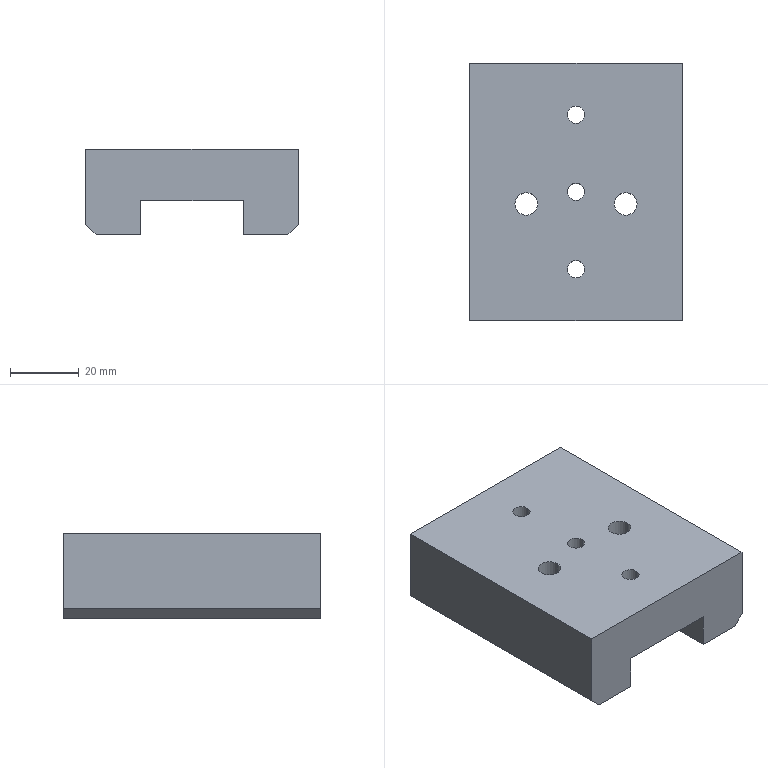Part | SolidWorks | features HoleWzd 3, Chamfer 1, Extrusion 1, ICE 1 | 1 solid | 30 faces | box 62 x 75 x 25 mm | volume 89108 mm3 | plane 16 | cylinder 14 | commonest cylinder face diameters 5 x6 6.6 x4 11 x4
STEP:
#1=CARTESIAN_POINT('',(17.8,-3.5,12.5));
#2=VERTEX_POINT('',#1);
#3=CARTESIAN_POINT('',(11.2,-3.5,12.5));
#4=VERTEX_POINT('',#3);
#5=CARTESIAN_POINT('',(14.5,-3.5,12.5));
#6=DIRECTION('',(0.,0.,-1.));
#7=DIRECTION('',(-1.,0.,0.));
#8=AXIS2_PLACEMENT_3D('',#5,#6,#7);
#9=CIRCLE('',#8,3.3);
#10=EDGE_CURVE('',#2,#4,#9,.T.);
#11=ORIENTED_EDGE('',*,*,#10,.F.);
#12=CARTESIAN_POINT('',(17.8,-3.5,7.5));
#13=VERTEX_POINT('',#12);
#14=CARTESIAN_POINT('',(17.8,-3.5,-12.5));
#15=DIRECTION('',(0.,0.,-1.));
#16=VECTOR('',#15,1000.);
#17=LINE('',#14,#16);
#18=EDGE_CURVE('',#2,#13,#17,.T.);
#19=ORIENTED_EDGE('',*,*,#18,.T.);
#20=CARTESIAN_POINT('',(11.2,-3.5,7.5));
#21=VERTEX_POINT('',#20);
#22=CARTESIAN_POINT('',(14.5,-3.5,7.5));
#23=DIRECTION('',(0.,0.,-1.));
#24=DIRECTION('',(-1.,0.,0.));
#25=AXIS2_PLACEMENT_3D('',#22,#23,#24);
#26=CIRCLE('',#25,3.3);
#27=EDGE_CURVE('',#13,#21,#26,.T.);
#28=ORIENTED_EDGE('',*,*,#27,.T.);
#29=CARTESIAN_POINT('',(11.2,-3.5,-12.5));
#30=DIRECTION('',(0.,0.,-1.));
#31=VECTOR('',#30,1000.);
#32=LINE('',#29,#31);
#33=EDGE_CURVE('',#4,#21,#32,.T.);
#34=ORIENTED_EDGE('',*,*,#33,.F.);
#35=EDGE_LOOP('',(#11,#19,#28,#34));
#36=FACE_OUTER_BOUND('',#35,.T.);
#37=CARTESIAN_POINT('',(14.5,-3.5,-12.5));
#38=DIRECTION('',(0.,0.,-1.));
#39=DIRECTION('',(-1.,0.,0.));
#40=AXIS2_PLACEMENT_3D('',#37,#38,#39);
#41=CYLINDRICAL_SURFACE('',#40,3.3);
#42=ADVANCED_FACE('',(#36),#41,.F.);
#43=CARTESIAN_POINT('',(20.,-3.5,7.5));
#44=VERTEX_POINT('',#43);
#45=CARTESIAN_POINT('',(9.,-3.5,7.5));
#46=VERTEX_POINT('',#45);
#47=CARTESIAN_POINT('',(14.5,-3.5,7.5));
#48=DIRECTION('',(0.,0.,-1.));
#49=DIRECTION('',(-1.,0.,0.));
#50=AXIS2_PLACEMENT_3D('',#47,#48,#49);
#51=CIRCLE('',#50,5.5);
#52=EDGE_CURVE('',#44,#46,#51,.T.);
#53=ORIENTED_EDGE('',*,*,#52,.F.);
#54=CARTESIAN_POINT('',(20.,-3.5,-12.5));
#55=VERTEX_POINT('',#54);
#56=CARTESIAN_POINT('',(20.,-3.5,-12.5));
#57=DIRECTION('',(0.,0.,-1.));
#58=VECTOR('',#57,1000.);
#59=LINE('',#56,#58);
#60=EDGE_CURVE('',#44,#55,#59,.T.);
#61=ORIENTED_EDGE('',*,*,#60,.T.);
#62=CARTESIAN_POINT('',(15.,-8.977,-12.5));
#63=VERTEX_POINT('',#62);
#64=CARTESIAN_POINT('',(14.5,-3.5,-12.5));
#65=DIRECTION('',(0.,0.,-1.));
#66=DIRECTION('',(-1.,0.,0.));
#67=AXIS2_PLACEMENT_3D('',#64,#65,#66);
#68=CIRCLE('',#67,5.5);
#69=EDGE_CURVE('',#55,#63,#68,.T.);
#70=ORIENTED_EDGE('',*,*,#69,.T.);
#71=CARTESIAN_POINT('',(15.,-8.977,-2.5));
#72=VERTEX_POINT('',#71);
#73=CARTESIAN_POINT('',(15.,-8.977,-12.5));
#74=DIRECTION('',(0.,0.,-1.));
#75=VECTOR('',#74,1000.);
#76=LINE('',#73,#75);
#77=EDGE_CURVE('',#72,#63,#76,.T.);
#78=ORIENTED_EDGE('',*,*,#77,.F.);
#79=CARTESIAN_POINT('',(9.,-3.5,-2.5));
#80=VERTEX_POINT('',#79);
#81=CARTESIAN_POINT('',(14.5,-3.5,-2.5));
#82=DIRECTION('',(0.,0.,-1.));
#83=DIRECTION('',(-1.,0.,0.));
#84=AXIS2_PLACEMENT_3D('',#81,#82,#83);
#85=CIRCLE('',#84,5.5);
#86=EDGE_CURVE('',#72,#80,#85,.T.);
#87=ORIENTED_EDGE('',*,*,#86,.T.);
#88=CARTESIAN_POINT('',(9.,-3.5,-12.5));
#89=DIRECTION('',(0.,0.,-1.));
#90=VECTOR('',#89,1000.);
#91=LINE('',#88,#90);
#92=EDGE_CURVE('',#46,#80,#91,.T.);
#93=ORIENTED_EDGE('',*,*,#92,.F.);
#94=EDGE_LOOP('',(#53,#61,#70,#78,#87,#93));
#95=FACE_OUTER_BOUND('',#94,.T.);
#96=CARTESIAN_POINT('',(14.5,-3.5,-12.5));
#97=DIRECTION('',(0.,0.,-1.));
#98=DIRECTION('',(-1.,0.,0.));
#99=AXIS2_PLACEMENT_3D('',#96,#97,#98);
#100=CYLINDRICAL_SURFACE('',#99,5.5);
#101=ADVANCED_FACE('',(#95),#100,.F.);
#102=CARTESIAN_POINT('',(-11.2,-3.5,12.5));
#103=VERTEX_POINT('',#102);
#104=CARTESIAN_POINT('',(-17.8,-3.5,12.5));
#105=VERTEX_POINT('',#104);
#106=CARTESIAN_POINT('',(-14.5,-3.5,12.5));
#107=DIRECTION('',(0.,0.,-1.));
#108=DIRECTION('',(-1.,0.,0.));
#109=AXIS2_PLACEMENT_3D('',#106,#107,#108);
#110=CIRCLE('',#109,3.3);
#111=EDGE_CURVE('',#103,#105,#110,.T.);
#112=ORIENTED_EDGE('',*,*,#111,.F.);
#113=CARTESIAN_POINT('',(-11.2,-3.5,7.5));
#114=VERTEX_POINT('',#113);
#115=CARTESIAN_POINT('',(-11.2,-3.5,-12.5));
#116=DIRECTION('',(0.,0.,-1.));
#117=VECTOR('',#116,1000.);
#118=LINE('',#115,#117);
#119=EDGE_CURVE('',#103,#114,#118,.T.);
#120=ORIENTED_EDGE('',*,*,#119,.T.);
#121=CARTESIAN_POINT('',(-17.8,-3.5,7.5));
#122=VERTEX_POINT('',#121);
#123=CARTESIAN_POINT('',(-14.5,-3.5,7.5));
#124=DIRECTION('',(0.,0.,-1.));
#125=DIRECTION('',(-1.,0.,0.));
#126=AXIS2_PLACEMENT_3D('',#123,#124,#125);
#127=CIRCLE('',#126,3.3);
#128=EDGE_CURVE('',#114,#122,#127,.T.);
#129=ORIENTED_EDGE('',*,*,#128,.T.);
#130=CARTESIAN_POINT('',(-17.8,-3.5,-12.5));
#131=DIRECTION('',(0.,0.,-1.));
#132=VECTOR('',#131,1000.);
#133=LINE('',#130,#132);
#134=EDGE_CURVE('',#105,#122,#133,.T.);
#135=ORIENTED_EDGE('',*,*,#134,.F.);
#136=EDGE_LOOP('',(#112,#120,#129,#135));
#137=FACE_OUTER_BOUND('',#136,.T.);
#138=CARTESIAN_POINT('',(-14.5,-3.5,-12.5));
#139=DIRECTION('',(0.,0.,-1.));
#140=DIRECTION('',(-1.,0.,0.));
#141=AXIS2_PLACEMENT_3D('',#138,#139,#140);
#142=CYLINDRICAL_SURFACE('',#141,3.3);
#143=ADVANCED_FACE('',(#137),#142,.F.);
#144=CARTESIAN_POINT('',(-9.,-3.5,7.5));
#145=VERTEX_POINT('',#144);
#146=CARTESIAN_POINT('',(-20.,-3.5,7.5));
#147=VERTEX_POINT('',#146);
#148=CARTESIAN_POINT('',(-14.5,-3.5,7.5));
#149=DIRECTION('',(0.,0.,-1.));
#150=DIRECTION('',(-1.,0.,0.));
#151=AXIS2_PLACEMENT_3D('',#148,#149,#150);
#152=CIRCLE('',#151,5.5);
#153=EDGE_CURVE('',#145,#147,#152,.T.);
#154=ORIENTED_EDGE('',*,*,#153,.F.);
#155=CARTESIAN_POINT('',(-9.,-3.5,-2.5));
#156=VERTEX_POINT('',#155);
#157=CARTESIAN_POINT('',(-9.,-3.5,-12.5));
#158=DIRECTION('',(0.,0.,-1.));
#159=VECTOR('',#158,1000.);
#160=LINE('',#157,#159);
#161=EDGE_CURVE('',#145,#156,#160,.T.);
#162=ORIENTED_EDGE('',*,*,#161,.T.);
#163=CARTESIAN_POINT('',(-15.,-8.977,-2.5));
#164=VERTEX_POINT('',#163);
#165=CARTESIAN_POINT('',(-14.5,-3.5,-2.5));
#166=DIRECTION('',(0.,0.,-1.));
#167=DIRECTION('',(-1.,0.,0.));
#168=AXIS2_PLACEMENT_3D('',#165,#166,#167);
#169=CIRCLE('',#168,5.5);
#170=EDGE_CURVE('',#156,#164,#169,.T.);
#171=ORIENTED_EDGE('',*,*,#170,.T.);
#172=CARTESIAN_POINT('',(-15.,-8.977,-12.5));
#173=VERTEX_POINT('',#172);
#174=CARTESIAN_POINT('',(-15.,-8.977,-12.5));
#175=DIRECTION('',(0.,0.,1.));
#176=VECTOR('',#175,1000.);
#177=LINE('',#174,#176);
#178=EDGE_CURVE('',#173,#164,#177,.T.);
#179=ORIENTED_EDGE('',*,*,#178,.F.);
#180=CARTESIAN_POINT('',(-20.,-3.5,-12.5));
#181=VERTEX_POINT('',#180);
#182=CARTESIAN_POINT('',(-14.5,-3.5,-12.5));
#183=DIRECTION('',(0.,0.,-1.));
#184=DIRECTION('',(-1.,0.,0.));
#185=AXIS2_PLACEMENT_3D('',#182,#183,#184);
#186=CIRCLE('',#185,5.5);
#187=EDGE_CURVE('',#173,#181,#186,.T.);
#188=ORIENTED_EDGE('',*,*,#187,.T.);
#189=CARTESIAN_POINT('',(-20.,-3.5,-12.5));
#190=DIRECTION('',(0.,0.,-1.));
#191=VECTOR('',#190,1000.);
#192=LINE('',#189,#191);
#193=EDGE_CURVE('',#147,#181,#192,.T.);
#194=ORIENTED_EDGE('',*,*,#193,.F.);
#195=EDGE_LOOP('',(#154,#162,#171,#179,#188,#194));
#196=FACE_OUTER_BOUND('',#195,.T.);
#197=CARTESIAN_POINT('',(-14.5,-3.5,-12.5));
#198=DIRECTION('',(0.,0.,-1.));
#199=DIRECTION('',(-1.,0.,0.));
#200=AXIS2_PLACEMENT_3D('',#197,#198,#199);
#201=CYLINDRICAL_SURFACE('',#200,5.5);
#202=ADVANCED_FACE('',(#196),#201,.F.);
#203=CARTESIAN_POINT('',(2.5,22.5,12.5));
#204=VERTEX_POINT('',#203);
#205=CARTESIAN_POINT('',(-2.5,22.5,12.5));
#206=VERTEX_POINT('',#205);
#207=CARTESIAN_POINT('',(0.,22.5,12.5));
#208=DIRECTION('',(0.,0.,-1.));
#209=DIRECTION('',(-1.,0.,0.));
#210=AXIS2_PLACEMENT_3D('',#207,#208,#209);
#211=CIRCLE('',#210,2.5);
#212=EDGE_CURVE('',#204,#206,#211,.T.);
#213=ORIENTED_EDGE('',*,*,#212,.F.);
#214=CARTESIAN_POINT('',(2.5,22.5,-2.5));
#215=VERTEX_POINT('',#214);
#216=CARTESIAN_POINT('',(2.5,22.5,-2.5));
#217=DIRECTION('',(0.,0.,-1.));
#218=VECTOR('',#217,1000.);
#219=LINE('',#216,#218);
#220=EDGE_CURVE('',#204,#215,#219,.T.);
#221=ORIENTED_EDGE('',*,*,#220,.T.);
#222=CARTESIAN_POINT('',(-2.5,22.5,-2.5));
#223=VERTEX_POINT('',#222);
#224=CARTESIAN_POINT('',(0.,22.5,-2.5));
#225=DIRECTION('',(0.,0.,-1.));
#226=DIRECTION('',(-1.,0.,0.));
#227=AXIS2_PLACEMENT_3D('',#224,#225,#226);
#228=CIRCLE('',#227,2.5);
#229=EDGE_CURVE('',#215,#223,#228,.T.);
#230=ORIENTED_EDGE('',*,*,#229,.T.);
#231=CARTESIAN_POINT('',(-2.5,22.5,-2.5));
#232=DIRECTION('',(0.,0.,-1.));
#233=VECTOR('',#232,1000.);
#234=LINE('',#231,#233);
#235=EDGE_CURVE('',#206,#223,#234,.T.);
#236=ORIENTED_EDGE('',*,*,#235,.F.);
#237=EDGE_LOOP('',(#213,#221,#230,#236));
#238=FACE_OUTER_BOUND('',#237,.T.);
#239=CARTESIAN_POINT('',(0.,22.5,-2.5));
#240=DIRECTION('',(0.,0.,-1.));
#241=DIRECTION('',(-1.,0.,0.));
#242=AXIS2_PLACEMENT_3D('',#239,#240,#241);
#243=CYLINDRICAL_SURFACE('',#242,2.5);
#244=ADVANCED_FACE('',(#238),#243,.F.);
#245=CARTESIAN_POINT('',(2.5,-22.5,12.5));
#246=VERTEX_POINT('',#245);
#247=CARTESIAN_POINT('',(-2.5,-22.5,12.5));
#248=VERTEX_POINT('',#247);
#249=CARTESIAN_POINT('',(0.,-22.5,12.5));
#250=DIRECTION('',(0.,0.,-1.));
#251=DIRECTION('',(-1.,0.,0.));
#252=AXIS2_PLACEMENT_3D('',#249,#250,#251);
#253=CIRCLE('',#252,2.5);
#254=EDGE_CURVE('',#246,#248,#253,.T.);
#255=ORIENTED_EDGE('',*,*,#254,.F.);
#256=CARTESIAN_POINT('',(2.5,-22.5,-2.5));
#257=VERTEX_POINT('',#256);
#258=CARTESIAN_POINT('',(2.5,-22.5,-2.5));
#259=DIRECTION('',(0.,0.,-1.));
#260=VECTOR('',#259,1000.);
#261=LINE('',#258,#260);
#262=EDGE_CURVE('',#246,#257,#261,.T.);
#263=ORIENTED_EDGE('',*,*,#262,.T.);
#264=CARTESIAN_POINT('',(-2.5,-22.5,-2.5));
#265=VERTEX_POINT('',#264);
#266=CARTESIAN_POINT('',(0.,-22.5,-2.5));
#267=DIRECTION('',(0.,0.,-1.));
#268=DIRECTION('',(-1.,0.,0.));
#269=AXIS2_PLACEMENT_3D('',#266,#267,#268);
#270=CIRCLE('',#269,2.5);
#271=EDGE_CURVE('',#257,#265,#270,.T.);
#272=ORIENTED_EDGE('',*,*,#271,.T.);
#273=CARTESIAN_POINT('',(-2.5,-22.5,-2.5));
#274=DIRECTION('',(0.,0.,-1.));
#275=VECTOR('',#274,1000.);
#276=LINE('',#273,#275);
#277=EDGE_CURVE('',#248,#265,#276,.T.);
#278=ORIENTED_EDGE('',*,*,#277,.F.);
#279=EDGE_LOOP('',(#255,#263,#272,#278));
#280=FACE_OUTER_BOUND('',#279,.T.);
#281=CARTESIAN_POINT('',(0.,-22.5,-2.5));
#282=DIRECTION('',(0.,0.,-1.));
#283=DIRECTION('',(-1.,0.,0.));
#284=AXIS2_PLACEMENT_3D('',#281,#282,#283);
#285=CYLINDRICAL_SURFACE('',#284,2.5);
#286=ADVANCED_FACE('',(#280),#285,.F.);
#287=CARTESIAN_POINT('',(-2.5,0.,-2.5));
#288=VERTEX_POINT('',#287);
#289=CARTESIAN_POINT('',(2.5,0.,-2.5));
#290=VERTEX_POINT('',#289);
#291=CARTESIAN_POINT('',(0.,0.,-2.5));
#292=DIRECTION('',(0.,0.,1.));
#293=DIRECTION('',(-1.,0.,0.));
#294=AXIS2_PLACEMENT_3D('',#291,#292,#293);
#295=CIRCLE('',#294,2.5);
#296=EDGE_CURVE('',#288,#290,#295,.T.);
#297=ORIENTED_EDGE('',*,*,#296,.F.);
#298=CARTESIAN_POINT('',(-2.5,0.,12.5));
#299=VERTEX_POINT('',#298);
#300=CARTESIAN_POINT('',(-2.5,0.,12.5));
#301=DIRECTION('',(0.,0.,1.));
#302=VECTOR('',#301,1000.);
#303=LINE('',#300,#302);
#304=EDGE_CURVE('',#288,#299,#303,.T.);
#305=ORIENTED_EDGE('',*,*,#304,.T.);
#306=CARTESIAN_POINT('',(2.5,0.,12.5));
#307=VERTEX_POINT('',#306);
#308=CARTESIAN_POINT('',(0.,0.,12.5));
#309=DIRECTION('',(0.,0.,1.));
#310=DIRECTION('',(1.,0.,0.));
#311=AXIS2_PLACEMENT_3D('',#308,#309,#310);
#312=CIRCLE('',#311,2.5);
#313=EDGE_CURVE('',#299,#307,#312,.T.);
#314=ORIENTED_EDGE('',*,*,#313,.T.);
#315=CARTESIAN_POINT('',(2.5,0.,12.5));
#316=DIRECTION('',(0.,0.,1.));
#317=VECTOR('',#316,1000.);
#318=LINE('',#315,#317);
#319=EDGE_CURVE('',#290,#307,#318,.T.);
#320=ORIENTED_EDGE('',*,*,#319,.F.);
#321=EDGE_LOOP('',(#297,#305,#314,#320));
#322=FACE_OUTER_BOUND('',#321,.T.);
#323=CARTESIAN_POINT('',(0.,0.,12.5));
#324=DIRECTION('',(0.,0.,1.));
#325=DIRECTION('',(1.,0.,0.));
#326=AXIS2_PLACEMENT_3D('',#323,#324,#325);
#327=CYLINDRICAL_SURFACE('',#326,2.5);
#328=ADVANCED_FACE('',(#322),#327,.F.);
#329=CARTESIAN_POINT('',(15.,-37.5,-2.5));
#330=VERTEX_POINT('',#329);
#331=CARTESIAN_POINT('',(15.,37.5,-2.5));
#332=DIRECTION('',(0.,-1.,0.));
#333=VECTOR('',#332,1000.);
#334=LINE('',#331,#333);
#335=EDGE_CURVE('',#72,#330,#334,.T.);
#336=ORIENTED_EDGE('',*,*,#335,.F.);
#337=ORIENTED_EDGE('',*,*,#77,.T.);
#338=CARTESIAN_POINT('',(15.,-37.5,-12.5));
#339=VERTEX_POINT('',#338);
#340=CARTESIAN_POINT('',(15.,37.5,-12.5));
#341=DIRECTION('',(0.,-1.,0.));
#342=VECTOR('',#341,1000.);
#343=LINE('',#340,#342);
#344=EDGE_CURVE('',#63,#339,#343,.T.);
#345=ORIENTED_EDGE('',*,*,#344,.T.);
#346=CARTESIAN_POINT('',(15.,-37.5,-2.5));
#347=DIRECTION('',(0.,0.,-1.));
#348=VECTOR('',#347,1000.);
#349=LINE('',#346,#348);
#350=EDGE_CURVE('',#330,#339,#349,.T.);
#351=ORIENTED_EDGE('',*,*,#350,.F.);
#352=EDGE_LOOP('',(#336,#337,#345,#351));
#353=FACE_OUTER_BOUND('',#352,.T.);
#354=CARTESIAN_POINT('',(15.,37.5,-2.5));
#355=DIRECTION('',(1.,0.,0.));
#356=DIRECTION('',(0.,1.,0.));
#357=AXIS2_PLACEMENT_3D('',#354,#355,#356);
#358=PLANE('',#357);
#359=ADVANCED_FACE('',(#353),#358,.F.);
#360=CARTESIAN_POINT('',(-15.,1.977,-2.5));
#361=VERTEX_POINT('',#360);
#362=CARTESIAN_POINT('',(-15.,37.5,-2.5));
#363=VERTEX_POINT('',#362);
#364=CARTESIAN_POINT('',(-15.,37.5,-2.5));
#365=DIRECTION('',(0.,1.,0.));
#366=VECTOR('',#365,1000.);
#367=LINE('',#364,#366);
#368=EDGE_CURVE('',#361,#363,#367,.T.);
#369=ORIENTED_EDGE('',*,*,#368,.F.);
#370=CARTESIAN_POINT('',(-15.,1.977,-12.5));
#371=VERTEX_POINT('',#370);
#372=CARTESIAN_POINT('',(-15.,1.977,-12.5));
#373=DIRECTION('',(0.,0.,-1.));
#374=VECTOR('',#373,1000.);
#375=LINE('',#372,#374);
#376=EDGE_CURVE('',#361,#371,#375,.T.);
#377=ORIENTED_EDGE('',*,*,#376,.T.);
#378=CARTESIAN_POINT('',(-15.,37.5,-12.5));
#379=VERTEX_POINT('',#378);
#380=CARTESIAN_POINT('',(-15.,37.5,-12.5));
#381=DIRECTION('',(0.,1.,0.));
#382=VECTOR('',#381,1000.);
#383=LINE('',#380,#382);
#384=EDGE_CURVE('',#371,#379,#383,.T.);
#385=ORIENTED_EDGE('',*,*,#384,.T.);
#386=CARTESIAN_POINT('',(-15.,37.5,-2.5));
#387=DIRECTION('',(0.,0.,-1.));
#388=VECTOR('',#387,1000.);
#389=LINE('',#386,#388);
#390=EDGE_CURVE('',#363,#379,#389,.T.);
#391=ORIENTED_EDGE('',*,*,#390,.F.);
#392=EDGE_LOOP('',(#369,#377,#385,#391));
#393=FACE_OUTER_BOUND('',#392,.T.);
#394=CARTESIAN_POINT('',(-15.,37.5,-2.5));
#395=DIRECTION('',(-1.,0.,0.));
#396=DIRECTION('',(0.,-1.,0.));
#397=AXIS2_PLACEMENT_3D('',#394,#395,#396);
#398=PLANE('',#397);
#399=ADVANCED_FACE('',(#393),#398,.F.);
#400=ORIENTED_EDGE('',*,*,#344,.F.);
#401=ORIENTED_EDGE('',*,*,#69,.F.);
#402=CARTESIAN_POINT('',(15.,1.977,-12.5));
#403=VERTEX_POINT('',#402);
#404=CARTESIAN_POINT('',(14.5,-3.5,-12.5));
#405=DIRECTION('',(0.,0.,-1.));
#406=DIRECTION('',(-1.,0.,0.));
#407=AXIS2_PLACEMENT_3D('',#404,#405,#406);
#408=CIRCLE('',#407,5.5);
#409=EDGE_CURVE('',#403,#55,#408,.T.);
#410=ORIENTED_EDGE('',*,*,#409,.F.);
#411=CARTESIAN_POINT('',(15.,37.5,-12.5));
#412=VERTEX_POINT('',#411);
#413=CARTESIAN_POINT('',(15.,37.5,-12.5));
#414=DIRECTION('',(0.,-1.,0.));
#415=VECTOR('',#414,1000.);
#416=LINE('',#413,#415);
#417=EDGE_CURVE('',#412,#403,#416,.T.);
#418=ORIENTED_EDGE('',*,*,#417,.F.);
#419=CARTESIAN_POINT('',(28.,37.5,-12.5));
#420=VERTEX_POINT('',#419);
#421=CARTESIAN_POINT('',(-31.,37.5,-12.5));
#422=DIRECTION('',(-1.,0.,0.));
#423=VECTOR('',#422,1000.);
#424=LINE('',#421,#423);
#425=EDGE_CURVE('',#420,#412,#424,.T.);
#426=ORIENTED_EDGE('',*,*,#425,.F.);
#427=CARTESIAN_POINT('',(28.,-37.5,-12.5));
#428=VERTEX_POINT('',#427);
#429=CARTESIAN_POINT('',(28.,0.,-12.5));
#430=DIRECTION('',(0.,-1.,0.));
#431=VECTOR('',#430,1000.);
#432=LINE('',#429,#431);
#433=EDGE_CURVE('',#420,#428,#432,.T.);
#434=ORIENTED_EDGE('',*,*,#433,.T.);
#435=CARTESIAN_POINT('',(-31.,-37.5,-12.5));
#436=DIRECTION('',(1.,0.,0.));
#437=VECTOR('',#436,1000.);
#438=LINE('',#435,#437);
#439=EDGE_CURVE('',#339,#428,#438,.T.);
#440=ORIENTED_EDGE('',*,*,#439,.F.);
#441=EDGE_LOOP('',(#400,#401,#410,#418,#426,#434,#440));
#442=FACE_OUTER_BOUND('',#441,.T.);
#443=CARTESIAN_POINT('',(0.,0.,-12.5));
#444=DIRECTION('',(0.,0.,1.));
#445=DIRECTION('',(1.,0.,0.));
#446=AXIS2_PLACEMENT_3D('',#443,#444,#445);
#447=PLANE('',#446);
#448=ADVANCED_FACE('',(#442),#447,.F.);
#449=ORIENTED_EDGE('',*,*,#304,.F.);
#450=CARTESIAN_POINT('',(0.,0.,-2.5));
#451=DIRECTION('',(0.,0.,1.));
#452=DIRECTION('',(-1.,0.,0.));
#453=AXIS2_PLACEMENT_3D('',#450,#451,#452);
#454=CIRCLE('',#453,2.5);
#455=EDGE_CURVE('',#290,#288,#454,.T.);
#456=ORIENTED_EDGE('',*,*,#455,.F.);
#457=ORIENTED_EDGE('',*,*,#319,.T.);
#458=CARTESIAN_POINT('',(0.,0.,12.5));
#459=DIRECTION('',(0.,0.,1.));
#460=DIRECTION('',(1.,0.,0.));
#461=AXIS2_PLACEMENT_3D('',#458,#459,#460);
#462=CIRCLE('',#461,2.5);
#463=EDGE_CURVE('',#307,#299,#462,.T.);
#464=ORIENTED_EDGE('',*,*,#463,.T.);
#465=EDGE_LOOP('',(#449,#456,#457,#464));
#466=FACE_OUTER_BOUND('',#465,.T.);
#467=CARTESIAN_POINT('',(0.,0.,12.5));
#468=DIRECTION('',(0.,0.,1.));
#469=DIRECTION('',(1.,0.,0.));
#470=AXIS2_PLACEMENT_3D('',#467,#468,#469);
#471=CYLINDRICAL_SURFACE('',#470,2.5);
#472=ADVANCED_FACE('',(#466),#471,.F.);
#473=CARTESIAN_POINT('',(31.,-37.5,12.5));
#474=VERTEX_POINT('',#473);
#475=CARTESIAN_POINT('',(31.,-37.5,-9.5));
#476=VERTEX_POINT('',#475);
#477=CARTESIAN_POINT('',(31.,-37.5,12.5));
#478=DIRECTION('',(0.,0.,-1.));
#479=VECTOR('',#478,1000.);
#480=LINE('',#477,#479);
#481=EDGE_CURVE('',#474,#476,#480,.T.);
#482=ORIENTED_EDGE('',*,*,#481,.T.);
#483=CARTESIAN_POINT('',(31.,37.5,-9.5));
#484=VERTEX_POINT('',#483);
#485=CARTESIAN_POINT('',(31.,37.5,-9.5));
#486=DIRECTION('',(0.,1.,0.));
#487=VECTOR('',#486,1000.);
#488=LINE('',#485,#487);
#489=EDGE_CURVE('',#476,#484,#488,.T.);
#490=ORIENTED_EDGE('',*,*,#489,.T.);
#491=CARTESIAN_POINT('',(31.,37.5,12.5));
#492=VERTEX_POINT('',#491);
#493=CARTESIAN_POINT('',(31.,37.5,12.5));
#494=DIRECTION('',(0.,0.,-1.));
#495=VECTOR('',#494,1000.);
#496=LINE('',#493,#495);
#497=EDGE_CURVE('',#492,#484,#496,.T.);
#498=ORIENTED_EDGE('',*,*,#497,.F.);
#499=CARTESIAN_POINT('',(31.,37.5,12.5));
#500=DIRECTION('',(0.,1.,0.));
#501=VECTOR('',#500,1000.);
#502=LINE('',#499,#501);
#503=EDGE_CURVE('',#474,#492,#502,.T.);
#504=ORIENTED_EDGE('',*,*,#503,.F.);
#505=EDGE_LOOP('',(#482,#490,#498,#504));
#506=FACE_OUTER_BOUND('',#505,.T.);
#507=CARTESIAN_POINT('',(31.,37.5,12.5));
#508=DIRECTION('',(-1.,0.,0.));
#509=DIRECTION('',(0.,-1.,0.));
#510=AXIS2_PLACEMENT_3D('',#507,#508,#509);
#511=PLANE('',#510);
#512=ADVANCED_FACE('',(#506),#511,.F.);
#513=ORIENTED_EDGE('',*,*,#425,.T.);
#514=CARTESIAN_POINT('',(15.,37.5,-2.5));
#515=VERTEX_POINT('',#514);
#516=CARTESIAN_POINT('',(15.,37.5,-2.5));
#517=DIRECTION('',(0.,0.,-1.));
#518=VECTOR('',#517,1000.);
#519=LINE('',#516,#518);
#520=EDGE_CURVE('',#515,#412,#519,.T.);
#521=ORIENTED_EDGE('',*,*,#520,.F.);
#522=CARTESIAN_POINT('',(15.,37.5,-2.5));
#523=DIRECTION('',(1.,0.,0.));
#524=VECTOR('',#523,1000.);
#525=LINE('',#522,#524);
#526=EDGE_CURVE('',#363,#515,#525,.T.);
#527=ORIENTED_EDGE('',*,*,#526,.F.);
#528=ORIENTED_EDGE('',*,*,#390,.T.);
#529=CARTESIAN_POINT('',(-28.,37.5,-12.5));
#530=VERTEX_POINT('',#529);
#531=CARTESIAN_POINT('',(-31.,37.5,-12.5));
#532=DIRECTION('',(-1.,0.,0.));
#533=VECTOR('',#532,1000.);
#534=LINE('',#531,#533);
#535=EDGE_CURVE('',#379,#530,#534,.T.);
#536=ORIENTED_EDGE('',*,*,#535,.T.);
#537=CARTESIAN_POINT('',(-31.,37.5,-9.5));
#538=VERTEX_POINT('',#537);
#539=CARTESIAN_POINT('',(-31.,37.5,-9.5));
#540=DIRECTION('',(-0.7071,0.,0.7071));
#541=VECTOR('',#540,1000.);
#542=LINE('',#539,#541);
#543=EDGE_CURVE('',#530,#538,#542,.T.);
#544=ORIENTED_EDGE('',*,*,#543,.T.);
#545=CARTESIAN_POINT('',(-31.,37.5,12.5));
#546=VERTEX_POINT('',#545);
#547=CARTESIAN_POINT('',(-31.,37.5,12.5));
#548=DIRECTION('',(0.,0.,-1.));
#549=VECTOR('',#548,1000.);
#550=LINE('',#547,#549);
#551=EDGE_CURVE('',#546,#538,#550,.T.);
#552=ORIENTED_EDGE('',*,*,#551,.F.);
#553=CARTESIAN_POINT('',(-31.,37.5,12.5));
#554=DIRECTION('',(-1.,0.,0.));
#555=VECTOR('',#554,1000.);
#556=LINE('',#553,#555);
#557=EDGE_CURVE('',#492,#546,#556,.T.);
#558=ORIENTED_EDGE('',*,*,#557,.F.);
#559=ORIENTED_EDGE('',*,*,#497,.T.);
#560=CARTESIAN_POINT('',(31.,37.5,-9.5));
#561=DIRECTION('',(-0.7071,0.,-0.7071));
#562=VECTOR('',#561,1000.);
#563=LINE('',#560,#562);
#564=EDGE_CURVE('',#484,#420,#563,.T.);
#565=ORIENTED_EDGE('',*,*,#564,.T.);
#566=EDGE_LOOP('',(#513,#521,#527,#528,#536,#544,#552,#558,#559,#565));
#567=FACE_OUTER_BOUND('',#566,.T.);
#568=CARTESIAN_POINT('',(-31.,37.5,12.5));
#569=DIRECTION('',(0.,-1.,0.));
#570=DIRECTION('',(0.,0.,-1.));
#571=AXIS2_PLACEMENT_3D('',#568,#569,#570);
#572=PLANE('',#571);
#573=ADVANCED_FACE('',(#567),#572,.F.);
#574=ORIENTED_EDGE('',*,*,#551,.T.);
#575=CARTESIAN_POINT('',(-31.,-37.5,-9.5));
#576=VERTEX_POINT('',#575);
#577=CARTESIAN_POINT('',(-31.,37.5,-9.5));
#578=DIRECTION('',(0.,-1.,0.));
#579=VECTOR('',#578,1000.);
#580=LINE('',#577,#579);
#581=EDGE_CURVE('',#538,#576,#580,.T.);
#582=ORIENTED_EDGE('',*,*,#581,.T.);
#583=CARTESIAN_POINT('',(-31.,-37.5,12.5));
#584=VERTEX_POINT('',#583);
#585=CARTESIAN_POINT('',(-31.,-37.5,12.5));
#586=DIRECTION('',(0.,0.,-1.));
#587=VECTOR('',#586,1000.);
#588=LINE('',#585,#587);
#589=EDGE_CURVE('',#584,#576,#588,.T.);
#590=ORIENTED_EDGE('',*,*,#589,.F.);
#591=CARTESIAN_POINT('',(-31.,37.5,12.5));
#592=DIRECTION('',(0.,-1.,0.));
#593=VECTOR('',#592,1000.);
#594=LINE('',#591,#593);
#595=EDGE_CURVE('',#546,#584,#594,.T.);
#596=ORIENTED_EDGE('',*,*,#595,.F.);
#597=EDGE_LOOP('',(#574,#582,#590,#596));
#598=FACE_OUTER_BOUND('',#597,.T.);
#599=CARTESIAN_POINT('',(-31.,37.5,12.5));
#600=DIRECTION('',(1.,0.,0.));
#601=DIRECTION('',(0.,1.,0.));
#602=AXIS2_PLACEMENT_3D('',#599,#600,#601);
#603=PLANE('',#602);
#604=ADVANCED_FACE('',(#598),#603,.F.);
#605=CARTESIAN_POINT('',(-15.,-37.5,-2.5));
#606=VERTEX_POINT('',#605);
#607=CARTESIAN_POINT('',(15.,-37.5,-2.5));
#608=DIRECTION('',(-1.,0.,0.));
#609=VECTOR('',#608,1000.);
#610=LINE('',#607,#609);
#611=EDGE_CURVE('',#330,#606,#610,.T.);
#612=ORIENTED_EDGE('',*,*,#611,.F.);
#613=ORIENTED_EDGE('',*,*,#350,.T.);
#614=ORIENTED_EDGE('',*,*,#439,.T.);
#615=CARTESIAN_POINT('',(31.,-37.5,-9.5));
#616=DIRECTION('',(0.7071,0.,0.7071));
#617=VECTOR('',#616,1000.);
#618=LINE('',#615,#617);
#619=EDGE_CURVE('',#428,#476,#618,.T.);
#620=ORIENTED_EDGE('',*,*,#619,.T.);
#621=ORIENTED_EDGE('',*,*,#481,.F.);
#622=CARTESIAN_POINT('',(-31.,-37.5,12.5));
#623=DIRECTION('',(1.,0.,0.));
#624=VECTOR('',#623,1000.);
#625=LINE('',#622,#624);
#626=EDGE_CURVE('',#584,#474,#625,.T.);
#627=ORIENTED_EDGE('',*,*,#626,.F.);
#628=ORIENTED_EDGE('',*,*,#589,.T.);
#629=CARTESIAN_POINT('',(-28.,-37.5,-12.5));
#630=VERTEX_POINT('',#629);
#631=CARTESIAN_POINT('',(-31.,-37.5,-9.5));
#632=DIRECTION('',(0.7071,0.,-0.7071));
#633=VECTOR('',#632,1000.);
#634=LINE('',#631,#633);
#635=EDGE_CURVE('',#576,#630,#634,.T.);
#636=ORIENTED_EDGE('',*,*,#635,.T.);
#637=CARTESIAN_POINT('',(-15.,-37.5,-12.5));
#638=VERTEX_POINT('',#637);
#639=CARTESIAN_POINT('',(-31.,-37.5,-12.5));
#640=DIRECTION('',(1.,0.,0.));
#641=VECTOR('',#640,1000.);
#642=LINE('',#639,#641);
#643=EDGE_CURVE('',#630,#638,#642,.T.);
#644=ORIENTED_EDGE('',*,*,#643,.T.);
#645=CARTESIAN_POINT('',(-15.,-37.5,-2.5));
#646=DIRECTION('',(0.,0.,-1.));
#647=VECTOR('',#646,1000.);
#648=LINE('',#645,#647);
#649=EDGE_CURVE('',#606,#638,#648,.T.);
#650=ORIENTED_EDGE('',*,*,#649,.F.);
#651=EDGE_LOOP('',(#612,#613,#614,#620,#621,#627,#628,#636,#644,#650));
#652=FACE_OUTER_BOUND('',#651,.T.);
#653=CARTESIAN_POINT('',(-31.,-37.5,12.5));
#654=DIRECTION('',(0.,1.,0.));
#655=DIRECTION('',(0.,0.,1.));
#656=AXIS2_PLACEMENT_3D('',#653,#654,#655);
#657=PLANE('',#656);
#658=ADVANCED_FACE('',(#652),#657,.F.);
#659=CARTESIAN_POINT('',(14.5,-3.5,12.5));
#660=DIRECTION('',(0.,0.,-1.));
#661=DIRECTION('',(-1.,0.,0.));
#662=AXIS2_PLACEMENT_3D('',#659,#660,#661);
#663=CIRCLE('',#662,3.3);
#664=EDGE_CURVE('',#4,#2,#663,.T.);
#665=ORIENTED_EDGE('',*,*,#664,.T.);
#666=ORIENTED_EDGE('',*,*,#10,.T.);
#667=EDGE_LOOP('',(#665,#666));
#668=FACE_BOUND('',#667,.T.);
#669=CARTESIAN_POINT('',(-14.5,-3.5,12.5));
#670=DIRECTION('',(0.,0.,-1.));
#671=DIRECTION('',(-1.,0.,0.));
#672=AXIS2_PLACEMENT_3D('',#669,#670,#671);
#673=CIRCLE('',#672,3.3);
#674=EDGE_CURVE('',#105,#103,#673,.T.);
#675=ORIENTED_EDGE('',*,*,#674,.T.);
#676=ORIENTED_EDGE('',*,*,#111,.T.);
#677=EDGE_LOOP('',(#675,#676));
#678=FACE_BOUND('',#677,.T.);
#679=CARTESIAN_POINT('',(0.,22.5,12.5));
#680=DIRECTION('',(0.,0.,-1.));
#681=DIRECTION('',(-1.,0.,0.));
#682=AXIS2_PLACEMENT_3D('',#679,#680,#681);
#683=CIRCLE('',#682,2.5);
#684=EDGE_CURVE('',#206,#204,#683,.T.);
#685=ORIENTED_EDGE('',*,*,#684,.T.);
#686=ORIENTED_EDGE('',*,*,#212,.T.);
#687=EDGE_LOOP('',(#685,#686));
#688=FACE_BOUND('',#687,.T.);
#689=CARTESIAN_POINT('',(0.,-22.5,12.5));
#690=DIRECTION('',(0.,0.,-1.));
#691=DIRECTION('',(-1.,0.,0.));
#692=AXIS2_PLACEMENT_3D('',#689,#690,#691);
#693=CIRCLE('',#692,2.5);
#694=EDGE_CURVE('',#248,#246,#693,.T.);
#695=ORIENTED_EDGE('',*,*,#694,.T.);
#696=ORIENTED_EDGE('',*,*,#254,.T.);
#697=EDGE_LOOP('',(#695,#696));
#698=FACE_BOUND('',#697,.T.);
#699=ORIENTED_EDGE('',*,*,#463,.F.);
#700=ORIENTED_EDGE('',*,*,#313,.F.);
#701=EDGE_LOOP('',(#699,#700));
#702=FACE_BOUND('',#701,.T.);
#703=ORIENTED_EDGE('',*,*,#503,.T.);
#704=ORIENTED_EDGE('',*,*,#557,.T.);
#705=ORIENTED_EDGE('',*,*,#595,.T.);
#706=ORIENTED_EDGE('',*,*,#626,.T.);
#707=EDGE_LOOP('',(#703,#704,#705,#706));
#708=FACE_OUTER_BOUND('',#707,.T.);
#709=CARTESIAN_POINT('',(0.,0.,12.5));
#710=DIRECTION('',(0.,0.,1.));
#711=DIRECTION('',(1.,0.,0.));
#712=AXIS2_PLACEMENT_3D('',#709,#710,#711);
#713=PLANE('',#712);
#714=ADVANCED_FACE('',(#668,#678,#688,#698,#702,#708),#713,.T.);
#715=ORIENTED_EDGE('',*,*,#384,.F.);
#716=CARTESIAN_POINT('',(-14.5,-3.5,-12.5));
#717=DIRECTION('',(0.,0.,-1.));
#718=DIRECTION('',(-1.,0.,0.));
#719=AXIS2_PLACEMENT_3D('',#716,#717,#718);
#720=CIRCLE('',#719,5.5);
#721=EDGE_CURVE('',#181,#371,#720,.T.);
#722=ORIENTED_EDGE('',*,*,#721,.F.);
#723=ORIENTED_EDGE('',*,*,#187,.F.);
#724=CARTESIAN_POINT('',(-15.,37.5,-12.5));
#725=DIRECTION('',(0.,1.,0.));
#726=VECTOR('',#725,1000.);
#727=LINE('',#724,#726);
#728=EDGE_CURVE('',#638,#173,#727,.T.);
#729=ORIENTED_EDGE('',*,*,#728,.F.);
#730=ORIENTED_EDGE('',*,*,#643,.F.);
#731=CARTESIAN_POINT('',(-28.,0.,-12.5));
#732=DIRECTION('',(0.,1.,0.));
#733=VECTOR('',#732,1000.);
#734=LINE('',#731,#733);
#735=EDGE_CURVE('',#630,#530,#734,.T.);
#736=ORIENTED_EDGE('',*,*,#735,.T.);
#737=ORIENTED_EDGE('',*,*,#535,.F.);
#738=EDGE_LOOP('',(#715,#722,#723,#729,#730,#736,#737));
#739=FACE_OUTER_BOUND('',#738,.T.);
#740=CARTESIAN_POINT('',(0.,0.,-12.5));
#741=DIRECTION('',(0.,0.,1.));
#742=DIRECTION('',(1.,0.,0.));
#743=AXIS2_PLACEMENT_3D('',#740,#741,#742);
#744=PLANE('',#743);
#745=ADVANCED_FACE('',(#739),#744,.F.);
#746=ORIENTED_EDGE('',*,*,#619,.F.);
#747=ORIENTED_EDGE('',*,*,#433,.F.);
#748=ORIENTED_EDGE('',*,*,#564,.F.);
#749=ORIENTED_EDGE('',*,*,#489,.F.);
#750=EDGE_LOOP('',(#746,#747,#748,#749));
#751=FACE_OUTER_BOUND('',#750,.T.);
#752=CARTESIAN_POINT('',(31.,37.5,-9.5));
#753=DIRECTION('',(-0.7071,0.,0.7071));
#754=DIRECTION('',(0.,1.,0.));
#755=AXIS2_PLACEMENT_3D('',#752,#753,#754);
#756=PLANE('',#755);
#757=ADVANCED_FACE('',(#751),#756,.F.);
#758=ORIENTED_EDGE('',*,*,#543,.F.);
#759=ORIENTED_EDGE('',*,*,#735,.F.);
#760=ORIENTED_EDGE('',*,*,#635,.F.);
#761=ORIENTED_EDGE('',*,*,#581,.F.);
#762=EDGE_LOOP('',(#758,#759,#760,#761));
#763=FACE_OUTER_BOUND('',#762,.T.);
#764=CARTESIAN_POINT('',(-31.,37.5,-9.5));
#765=DIRECTION('',(0.7071,0.,0.7071));
#766=DIRECTION('',(0.,-1.,0.));
#767=AXIS2_PLACEMENT_3D('',#764,#765,#766);
#768=PLANE('',#767);
#769=ADVANCED_FACE('',(#763),#768,.F.);
#770=ORIENTED_EDGE('',*,*,#86,.F.);
#771=ORIENTED_EDGE('',*,*,#335,.T.);
#772=ORIENTED_EDGE('',*,*,#611,.T.);
#773=CARTESIAN_POINT('',(-15.,37.5,-2.5));
#774=DIRECTION('',(0.,1.,0.));
#775=VECTOR('',#774,1000.);
#776=LINE('',#773,#775);
#777=EDGE_CURVE('',#606,#164,#776,.T.);
#778=ORIENTED_EDGE('',*,*,#777,.T.);
#779=ORIENTED_EDGE('',*,*,#170,.F.);
#780=CARTESIAN_POINT('',(-14.5,-3.5,-2.5));
#781=DIRECTION('',(0.,0.,-1.));
#782=DIRECTION('',(-1.,0.,0.));
#783=AXIS2_PLACEMENT_3D('',#780,#781,#782);
#784=CIRCLE('',#783,5.5);
#785=EDGE_CURVE('',#361,#156,#784,.T.);
#786=ORIENTED_EDGE('',*,*,#785,.F.);
#787=ORIENTED_EDGE('',*,*,#368,.T.);
#788=ORIENTED_EDGE('',*,*,#526,.T.);
#789=CARTESIAN_POINT('',(15.,1.977,-2.5));
#790=VERTEX_POINT('',#789);
#791=CARTESIAN_POINT('',(15.,37.5,-2.5));
#792=DIRECTION('',(0.,-1.,0.));
#793=VECTOR('',#792,1000.);
#794=LINE('',#791,#793);
#795=EDGE_CURVE('',#515,#790,#794,.T.);
#796=ORIENTED_EDGE('',*,*,#795,.T.);
#797=CARTESIAN_POINT('',(14.5,-3.5,-2.5));
#798=DIRECTION('',(0.,0.,-1.));
#799=DIRECTION('',(-1.,0.,0.));
#800=AXIS2_PLACEMENT_3D('',#797,#798,#799);
#801=CIRCLE('',#800,5.5);
#802=EDGE_CURVE('',#80,#790,#801,.T.);
#803=ORIENTED_EDGE('',*,*,#802,.F.);
#804=EDGE_LOOP('',(#770,#771,#772,#778,#779,#786,#787,#788,#796,#803));
#805=FACE_OUTER_BOUND('',#804,.T.);
#806=CARTESIAN_POINT('',(0.,22.5,-2.5));
#807=DIRECTION('',(0.,0.,-1.));
#808=DIRECTION('',(-1.,0.,0.));
#809=AXIS2_PLACEMENT_3D('',#806,#807,#808);
#810=CIRCLE('',#809,2.5);
#811=EDGE_CURVE('',#223,#215,#810,.T.);
#812=ORIENTED_EDGE('',*,*,#811,.F.);
#813=ORIENTED_EDGE('',*,*,#229,.F.);
#814=EDGE_LOOP('',(#812,#813));
#815=FACE_BOUND('',#814,.T.);
#816=CARTESIAN_POINT('',(0.,-22.5,-2.5));
#817=DIRECTION('',(0.,0.,-1.));
#818=DIRECTION('',(-1.,0.,0.));
#819=AXIS2_PLACEMENT_3D('',#816,#817,#818);
#820=CIRCLE('',#819,2.5);
#821=EDGE_CURVE('',#265,#257,#820,.T.);
#822=ORIENTED_EDGE('',*,*,#821,.F.);
#823=ORIENTED_EDGE('',*,*,#271,.F.);
#824=EDGE_LOOP('',(#822,#823));
#825=FACE_BOUND('',#824,.T.);
#826=ORIENTED_EDGE('',*,*,#455,.T.);
#827=ORIENTED_EDGE('',*,*,#296,.T.);
#828=EDGE_LOOP('',(#826,#827));
#829=FACE_BOUND('',#828,.T.);
#830=CARTESIAN_POINT('',(0.,0.,-2.5));
#831=DIRECTION('',(0.,0.,-1.));
#832=DIRECTION('',(-1.,0.,0.));
#833=AXIS2_PLACEMENT_3D('',#830,#831,#832);
#834=PLANE('',#833);
#835=ADVANCED_FACE('',(#805,#815,#825,#829),#834,.T.);
#836=ORIENTED_EDGE('',*,*,#417,.T.);
#837=CARTESIAN_POINT('',(15.,1.977,-12.5));
#838=DIRECTION('',(0.,0.,1.));
#839=VECTOR('',#838,1000.);
#840=LINE('',#837,#839);
#841=EDGE_CURVE('',#403,#790,#840,.T.);
#842=ORIENTED_EDGE('',*,*,#841,.T.);
#843=ORIENTED_EDGE('',*,*,#795,.F.);
#844=ORIENTED_EDGE('',*,*,#520,.T.);
#845=EDGE_LOOP('',(#836,#842,#843,#844));
#846=FACE_OUTER_BOUND('',#845,.T.);
#847=CARTESIAN_POINT('',(15.,37.5,-2.5));
#848=DIRECTION('',(1.,0.,0.));
#849=DIRECTION('',(0.,1.,0.));
#850=AXIS2_PLACEMENT_3D('',#847,#848,#849);
#851=PLANE('',#850);
#852=ADVANCED_FACE('',(#846),#851,.F.);
#853=ORIENTED_EDGE('',*,*,#728,.T.);
#854=ORIENTED_EDGE('',*,*,#178,.T.);
#855=ORIENTED_EDGE('',*,*,#777,.F.);
#856=ORIENTED_EDGE('',*,*,#649,.T.);
#857=EDGE_LOOP('',(#853,#854,#855,#856));
#858=FACE_OUTER_BOUND('',#857,.T.);
#859=CARTESIAN_POINT('',(-15.,37.5,-2.5));
#860=DIRECTION('',(-1.,0.,0.));
#861=DIRECTION('',(0.,-1.,0.));
#862=AXIS2_PLACEMENT_3D('',#859,#860,#861);
#863=PLANE('',#862);
#864=ADVANCED_FACE('',(#858),#863,.F.);
#865=ORIENTED_EDGE('',*,*,#262,.F.);
#866=ORIENTED_EDGE('',*,*,#694,.F.);
#867=ORIENTED_EDGE('',*,*,#277,.T.);
#868=ORIENTED_EDGE('',*,*,#821,.T.);
#869=EDGE_LOOP('',(#865,#866,#867,#868));
#870=FACE_OUTER_BOUND('',#869,.T.);
#871=CARTESIAN_POINT('',(0.,-22.5,-2.5));
#872=DIRECTION('',(0.,0.,-1.));
#873=DIRECTION('',(-1.,0.,0.));
#874=AXIS2_PLACEMENT_3D('',#871,#872,#873);
#875=CYLINDRICAL_SURFACE('',#874,2.5);
#876=ADVANCED_FACE('',(#870),#875,.F.);
#877=ORIENTED_EDGE('',*,*,#220,.F.);
#878=ORIENTED_EDGE('',*,*,#684,.F.);
#879=ORIENTED_EDGE('',*,*,#235,.T.);
#880=ORIENTED_EDGE('',*,*,#811,.T.);
#881=EDGE_LOOP('',(#877,#878,#879,#880));
#882=FACE_OUTER_BOUND('',#881,.T.);
#883=CARTESIAN_POINT('',(0.,22.5,-2.5));
#884=DIRECTION('',(0.,0.,-1.));
#885=DIRECTION('',(-1.,0.,0.));
#886=AXIS2_PLACEMENT_3D('',#883,#884,#885);
#887=CYLINDRICAL_SURFACE('',#886,2.5);
#888=ADVANCED_FACE('',(#882),#887,.F.);
#889=ORIENTED_EDGE('',*,*,#161,.F.);
#890=CARTESIAN_POINT('',(-14.5,-3.5,7.5));
#891=DIRECTION('',(0.,0.,-1.));
#892=DIRECTION('',(-1.,0.,0.));
#893=AXIS2_PLACEMENT_3D('',#890,#891,#892);
#894=CIRCLE('',#893,5.5);
#895=EDGE_CURVE('',#147,#145,#894,.T.);
#896=ORIENTED_EDGE('',*,*,#895,.F.);
#897=ORIENTED_EDGE('',*,*,#193,.T.);
#898=ORIENTED_EDGE('',*,*,#721,.T.);
#899=ORIENTED_EDGE('',*,*,#376,.F.);
#900=ORIENTED_EDGE('',*,*,#785,.T.);
#901=EDGE_LOOP('',(#889,#896,#897,#898,#899,#900));
#902=FACE_OUTER_BOUND('',#901,.T.);
#903=CARTESIAN_POINT('',(-14.5,-3.5,-12.5));
#904=DIRECTION('',(0.,0.,-1.));
#905=DIRECTION('',(-1.,0.,0.));
#906=AXIS2_PLACEMENT_3D('',#903,#904,#905);
#907=CYLINDRICAL_SURFACE('',#906,5.5);
#908=ADVANCED_FACE('',(#902),#907,.F.);
#909=ORIENTED_EDGE('',*,*,#119,.F.);
#910=ORIENTED_EDGE('',*,*,#674,.F.);
#911=ORIENTED_EDGE('',*,*,#134,.T.);
#912=CARTESIAN_POINT('',(-14.5,-3.5,7.5));
#913=DIRECTION('',(0.,0.,-1.));
#914=DIRECTION('',(-1.,0.,0.));
#915=AXIS2_PLACEMENT_3D('',#912,#913,#914);
#916=CIRCLE('',#915,3.3);
#917=EDGE_CURVE('',#122,#114,#916,.T.);
#918=ORIENTED_EDGE('',*,*,#917,.T.);
#919=EDGE_LOOP('',(#909,#910,#911,#918));
#920=FACE_OUTER_BOUND('',#919,.T.);
#921=CARTESIAN_POINT('',(-14.5,-3.5,-12.5));
#922=DIRECTION('',(0.,0.,-1.));
#923=DIRECTION('',(-1.,0.,0.));
#924=AXIS2_PLACEMENT_3D('',#921,#922,#923);
#925=CYLINDRICAL_SURFACE('',#924,3.3);
#926=ADVANCED_FACE('',(#920),#925,.F.);
#927=ORIENTED_EDGE('',*,*,#917,.F.);
#928=ORIENTED_EDGE('',*,*,#128,.F.);
#929=EDGE_LOOP('',(#927,#928));
#930=FACE_BOUND('',#929,.T.);
#931=ORIENTED_EDGE('',*,*,#895,.T.);
#932=ORIENTED_EDGE('',*,*,#153,.T.);
#933=EDGE_LOOP('',(#931,#932));
#934=FACE_OUTER_BOUND('',#933,.T.);
#935=CARTESIAN_POINT('',(-11.2,-3.5,7.5));
#936=DIRECTION('',(0.,0.,1.));
#937=DIRECTION('',(1.,0.,0.));
#938=AXIS2_PLACEMENT_3D('',#935,#936,#937);
#939=PLANE('',#938);
#940=ADVANCED_FACE('',(#930,#934),#939,.F.);
#941=ORIENTED_EDGE('',*,*,#60,.F.);
#942=CARTESIAN_POINT('',(14.5,-3.5,7.5));
#943=DIRECTION('',(0.,0.,-1.));
#944=DIRECTION('',(-1.,0.,0.));
#945=AXIS2_PLACEMENT_3D('',#942,#943,#944);
#946=CIRCLE('',#945,5.5);
#947=EDGE_CURVE('',#46,#44,#946,.T.);
#948=ORIENTED_EDGE('',*,*,#947,.F.);
#949=ORIENTED_EDGE('',*,*,#92,.T.);
#950=ORIENTED_EDGE('',*,*,#802,.T.);
#951=ORIENTED_EDGE('',*,*,#841,.F.);
#952=ORIENTED_EDGE('',*,*,#409,.T.);
#953=EDGE_LOOP('',(#941,#948,#949,#950,#951,#952));
#954=FACE_OUTER_BOUND('',#953,.T.);
#955=CARTESIAN_POINT('',(14.5,-3.5,-12.5));
#956=DIRECTION('',(0.,0.,-1.));
#957=DIRECTION('',(-1.,0.,0.));
#958=AXIS2_PLACEMENT_3D('',#955,#956,#957);
#959=CYLINDRICAL_SURFACE('',#958,5.5);
#960=ADVANCED_FACE('',(#954),#959,.F.);
#961=ORIENTED_EDGE('',*,*,#18,.F.);
#962=ORIENTED_EDGE('',*,*,#664,.F.);
#963=ORIENTED_EDGE('',*,*,#33,.T.);
#964=CARTESIAN_POINT('',(14.5,-3.5,7.5));
#965=DIRECTION('',(0.,0.,-1.));
#966=DIRECTION('',(-1.,0.,0.));
#967=AXIS2_PLACEMENT_3D('',#964,#965,#966);
#968=CIRCLE('',#967,3.3);
#969=EDGE_CURVE('',#21,#13,#968,.T.);
#970=ORIENTED_EDGE('',*,*,#969,.T.);
#971=EDGE_LOOP('',(#961,#962,#963,#970));
#972=FACE_OUTER_BOUND('',#971,.T.);
#973=CARTESIAN_POINT('',(14.5,-3.5,-12.5));
#974=DIRECTION('',(0.,0.,-1.));
#975=DIRECTION('',(-1.,0.,0.));
#976=AXIS2_PLACEMENT_3D('',#973,#974,#975);
#977=CYLINDRICAL_SURFACE('',#976,3.3);
#978=ADVANCED_FACE('',(#972),#977,.F.);
#979=ORIENTED_EDGE('',*,*,#969,.F.);
#980=ORIENTED_EDGE('',*,*,#27,.F.);
#981=EDGE_LOOP('',(#979,#980));
#982=FACE_BOUND('',#981,.T.);
#983=ORIENTED_EDGE('',*,*,#947,.T.);
#984=ORIENTED_EDGE('',*,*,#52,.T.);
#985=EDGE_LOOP('',(#983,#984));
#986=FACE_OUTER_BOUND('',#985,.T.);
#987=CARTESIAN_POINT('',(17.8,-3.5,7.5));
#988=DIRECTION('',(0.,0.,1.));
#989=DIRECTION('',(1.,0.,0.));
#990=AXIS2_PLACEMENT_3D('',#987,#988,#989);
#991=PLANE('',#990);
#992=ADVANCED_FACE('',(#982,#986),#991,.F.);
#993=CLOSED_SHELL('',(#42,#101,#143,#202,#244,#286,#328,#359,#399,#448,#472,#512,#573,#604,#658,#714,#745,#757,#769,#835,#852,#864,#876,#888,#908,#926,#940,#960,#978,#992));
#994=MANIFOLD_SOLID_BREP('',#993);
#995=CARTESIAN_POINT('',(0.,0.,0.));
#996=DIRECTION('',(0.,0.,1.));
#997=DIRECTION('',(1.,0.,0.));
#998=AXIS2_PLACEMENT_3D('',#995,#996,#997);
#999=(LENGTH_UNIT()NAMED_UNIT(*)SI_UNIT(.MILLI.,.METRE.));
#1000=UNCERTAINTY_MEASURE_WITH_UNIT(LENGTH_MEASURE(0.00001),#999,'','');
#1001=(NAMED_UNIT(*)PLANE_ANGLE_UNIT()SI_UNIT($,.RADIAN.));
#1002=(NAMED_UNIT(*)SI_UNIT($,.STERADIAN.)SOLID_ANGLE_UNIT());
#1003=(GEOMETRIC_REPRESENTATION_CONTEXT(3)GLOBAL_UNCERTAINTY_ASSIGNED_CONTEXT((#1000))GLOBAL_UNIT_ASSIGNED_CONTEXT((#999,#1001,#1002))REPRESENTATION_CONTEXT('',''));
#1004=ADVANCED_BREP_SHAPE_REPRESENTATION('',(#994,#998),#1003);